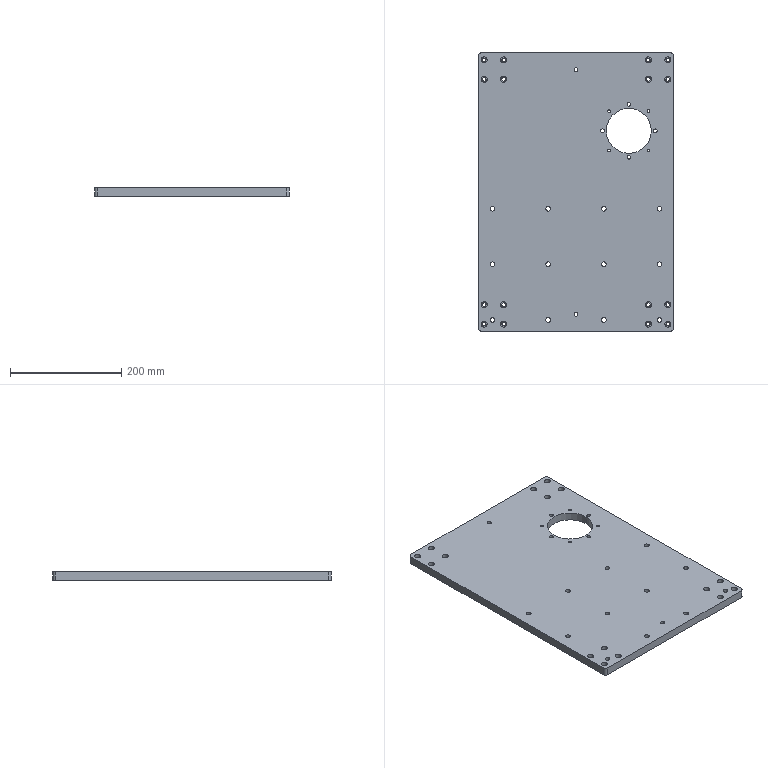CAM job | Mastercam | 3-axis milling, drilling | part box 350 x 500 x 15 mm | stock box 350 x 500 x 15 mm
Tools:
tool_number,name,type,diameter_mm,corner_radius_mm,flutes,flute_length_mm,overall_length_mm,shoulder_length_mm,holder_diameter_mm,length_offset,diameter_offset,default_rpm,default_feed_mm_min,default_plunge_mm_min,coolant
6,6 Flat End Mill,end mill,6,0,4,25,75,25,50,6,6,7000,3000,600,COOL_OFF
7,4 Chamfer Mill,chamfer mill,4,0,4,25,75,30,50,7,7,7000,1000,600,COOL_OFF
9,10 Flat End Mill,end mill,10,0,4,25,75,25,50,9,9,7000,3000,600,COOL_OFF
10,10 Flat End Mill,end mill,10,0,4,25,75,25,50,10,10,7000,1000,600,COOL_OFF
24,100 Flat End Mill,end mill,100,0,4,25,75,25,50,24,24,100,12,600,COOL_OFF
Operations:
seq,operation,operation_type,tool_number,tool_name,tool_diameter_mm,spindle_rpm,feed_mm_min,plunge_mm_min,retract_mm_min,cycle_time_s,wcs,posted,nc_file
1,Facing - [WCS: Plane-1] - [Tplane: Plane-1],Facing,24,100 Flat End Mill,100,4000,1000,600,1200,215.202,Plane-1,yes,.nc
2,Contour (Ramp) - [WCS: Plane-1] - [Tplane: Plane-1],Contour,9,10 Flat End Mill,10,7000,3000,600,1200,1066.202,Plane-1,yes,.nc
3,Contour (2D) - [WCS: Plane-1] - [Tplane: Plane-1],Contour,10,10 Flat End Mill,10,7000,1000,600,1200,106.3,Plane-1,yes,.nc
4,Contour (2D chamfer) - [WCS: Plane-1] - [Tplane: Plane-1],Contour,7,4 Chamfer Mill,4,7000,1000,600,1200,102.512,Plane-1,yes,.nc
5,Manual Entry (Cl),ManualEntry,,,,0,0,0,0,0,Plane-1,yes,.nc
6,Manual Entry (M00),ManualEntry,,,,0,0,0,0,0,Plane-1,yes,.nc
7,Helix Bore - [WCS: Plane-1] - [Tplane: Plane-1],HelixBore,6,6 Flat End Mill,6,7000,3000,600,1200,52.866,Plane-1,yes,.nc
8,Drill/Counterbore - [WCS: Plane-1] - [Tplane: Plane-1],Drill,7,4 Chamfer Mill,4,3000,300,600,1200,31.759,Plane-1,yes,.nc
9,Contour (2D chamfer) - [WCS: Plane-1] - [Tplane: Plane-1],Contour,7,4 Chamfer Mill,4,7000,1000,600,1200,10.443,Plane-1,yes,.nc
10,Helix Bore - [WCS: Plane] - [Tplane: Plane],HelixBore,6,6 Flat End Mill,6,7000,3000,600,1200,215.185,Plane,yes,.nc
11,Contour (Ramp) - [WCS: Plane] - [Tplane: Plane],Contour,6,6 Flat End Mill,6,7000,3000,600,1200,23.145,Plane,yes,.nc
12,Contour (2D chamfer) - [WCS: Plane] - [Tplane: Plane],Contour,7,4 Chamfer Mill,4,7000,1000,600,1200,160.091,Plane,yes,.nc
13,Manual Entry (M00),ManualEntry,,,,0,0,0,0,0,Plane,yes,.nc
14,Manual Entry (Cl),ManualEntry,,,,0,0,0,0,0,Plane,yes,.nc
15,Contour (Ramp) - [WCS: Plane] - [Tplane: Plane],Contour,6,6 Flat End Mill,6,7000,3000,600,1200,144.545,Plane,yes,.nc
16,Contour (Ramp) - [WCS: Plane] - [Tplane: Plane],Contour,6,6 Flat End Mill,6,7000,1000,600,1200,49.804,Plane,yes,.nc